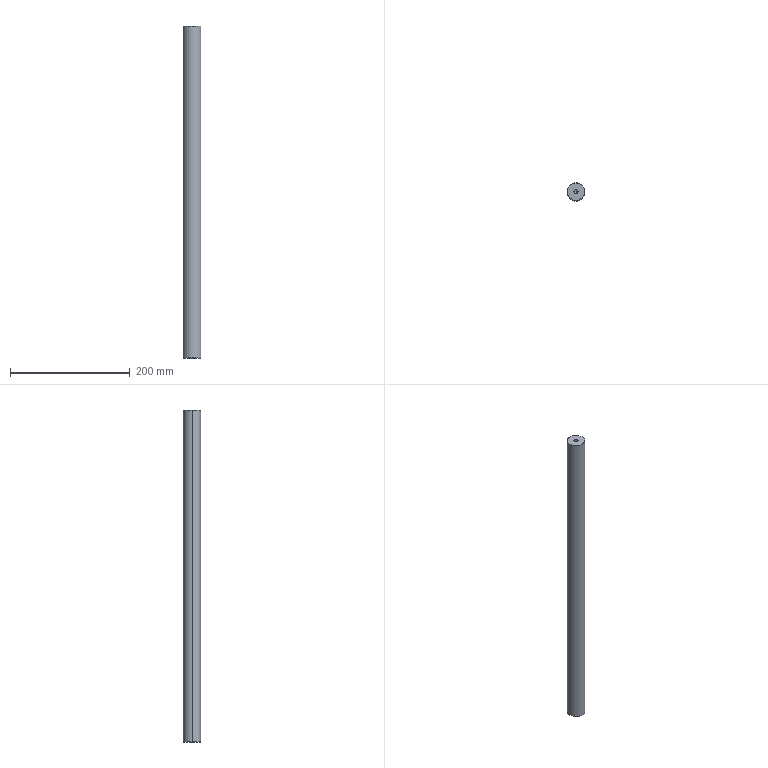Part | STEP file | 11-FG-SJ01511 | 1 solid | 16 faces | box 30 x 30 x 554 mm | volume 390089 mm3 | cone 8 | cylinder 6 | plane 2 | commonest cylinder face diameters 6.8 x4 30 x2
STEP:
#1=CARTESIAN_POINT('',(-14.5,0.,0.));
#2=VERTEX_POINT('',#1);
#3=CARTESIAN_POINT('',(14.5,0.,0.));
#4=VERTEX_POINT('',#3);
#5=CARTESIAN_POINT('',(0.,0.,0.));
#6=DIRECTION('',(0.,0.,-1.));
#7=DIRECTION('',(1.,0.,0.));
#8=AXIS2_PLACEMENT_3D('',#5,#6,#7);
#9=CIRCLE('',#8,14.5);
#10=EDGE_CURVE('',#2,#4,#9,.T.);
#11=ORIENTED_EDGE('',*,*,#10,.F.);
#12=CARTESIAN_POINT('',(-15.,0.,0.5));
#13=VERTEX_POINT('',#12);
#14=CARTESIAN_POINT('',(-15.,0.,0.5));
#15=DIRECTION('',(-0.7071,0.,0.7071));
#16=VECTOR('',#15,1000.);
#17=LINE('',#14,#16);
#18=EDGE_CURVE('',#2,#13,#17,.T.);
#19=ORIENTED_EDGE('',*,*,#18,.T.);
#20=CARTESIAN_POINT('',(15.,0.,0.5));
#21=VERTEX_POINT('',#20);
#22=CARTESIAN_POINT('',(0.,0.,0.5));
#23=DIRECTION('',(0.,0.,1.));
#24=DIRECTION('',(1.,0.,0.));
#25=AXIS2_PLACEMENT_3D('',#22,#23,#24);
#26=CIRCLE('',#25,15.);
#27=EDGE_CURVE('',#21,#13,#26,.T.);
#28=ORIENTED_EDGE('',*,*,#27,.F.);
#29=CARTESIAN_POINT('',(15.,0.,0.5));
#30=DIRECTION('',(0.7071,0.,0.7071));
#31=VECTOR('',#30,1000.);
#32=LINE('',#29,#31);
#33=EDGE_CURVE('',#4,#21,#32,.T.);
#34=ORIENTED_EDGE('',*,*,#33,.F.);
#35=EDGE_LOOP('',(#11,#19,#28,#34));
#36=FACE_OUTER_BOUND('',#35,.T.);
#37=CARTESIAN_POINT('',(0.,0.,0.5));
#38=DIRECTION('',(0.,0.,1.));
#39=DIRECTION('',(1.,0.,0.));
#40=AXIS2_PLACEMENT_3D('',#37,#38,#39);
#41=CONICAL_SURFACE('',#40,15.,0.7854);
#42=ADVANCED_FACE('',(#36),#41,.T.);
#43=CARTESIAN_POINT('',(14.5,0.,554.));
#44=VERTEX_POINT('',#43);
#45=CARTESIAN_POINT('',(-14.5,0.,554.));
#46=VERTEX_POINT('',#45);
#47=CARTESIAN_POINT('',(0.,0.,554.));
#48=DIRECTION('',(0.,0.,1.));
#49=DIRECTION('',(1.,0.,0.));
#50=AXIS2_PLACEMENT_3D('',#47,#48,#49);
#51=CIRCLE('',#50,14.5);
#52=EDGE_CURVE('',#44,#46,#51,.T.);
#53=ORIENTED_EDGE('',*,*,#52,.F.);
#54=CARTESIAN_POINT('',(15.,0.,553.5));
#55=VERTEX_POINT('',#54);
#56=CARTESIAN_POINT('',(14.5,0.,554.));
#57=DIRECTION('',(0.7071,0.,-0.7071));
#58=VECTOR('',#57,1000.);
#59=LINE('',#56,#58);
#60=EDGE_CURVE('',#44,#55,#59,.T.);
#61=ORIENTED_EDGE('',*,*,#60,.T.);
#62=CARTESIAN_POINT('',(-15.,0.,553.5));
#63=VERTEX_POINT('',#62);
#64=CARTESIAN_POINT('',(0.,0.,553.5));
#65=DIRECTION('',(0.,0.,-1.));
#66=DIRECTION('',(1.,0.,0.));
#67=AXIS2_PLACEMENT_3D('',#64,#65,#66);
#68=CIRCLE('',#67,15.);
#69=EDGE_CURVE('',#63,#55,#68,.T.);
#70=ORIENTED_EDGE('',*,*,#69,.F.);
#71=CARTESIAN_POINT('',(-14.5,0.,554.));
#72=DIRECTION('',(-0.7071,0.,-0.7071));
#73=VECTOR('',#72,1000.);
#74=LINE('',#71,#73);
#75=EDGE_CURVE('',#46,#63,#74,.T.);
#76=ORIENTED_EDGE('',*,*,#75,.F.);
#77=EDGE_LOOP('',(#53,#61,#70,#76));
#78=FACE_OUTER_BOUND('',#77,.T.);
#79=CARTESIAN_POINT('',(0.,0.,554.));
#80=DIRECTION('',(0.,0.,-1.));
#81=DIRECTION('',(-1.,0.,0.));
#82=AXIS2_PLACEMENT_3D('',#79,#80,#81);
#83=CONICAL_SURFACE('',#82,14.5,0.7854);
#84=ADVANCED_FACE('',(#78),#83,.T.);
#85=CARTESIAN_POINT('',(-3.4,0.,534.2));
#86=VERTEX_POINT('',#85);
#87=CARTESIAN_POINT('',(3.4,0.,534.2));
#88=VERTEX_POINT('',#87);
#89=CARTESIAN_POINT('',(0.,0.,534.2));
#90=DIRECTION('',(0.,0.,1.));
#91=DIRECTION('',(1.,0.,0.));
#92=AXIS2_PLACEMENT_3D('',#89,#90,#91);
#93=CIRCLE('',#92,3.4);
#94=EDGE_CURVE('',#86,#88,#93,.T.);
#95=ORIENTED_EDGE('',*,*,#94,.F.);
#96=CARTESIAN_POINT('',(-3.4,0.,554.));
#97=VERTEX_POINT('',#96);
#98=CARTESIAN_POINT('',(-3.4,0.,554.));
#99=DIRECTION('',(0.,0.,1.));
#100=VECTOR('',#99,1000.);
#101=LINE('',#98,#100);
#102=EDGE_CURVE('',#86,#97,#101,.T.);
#103=ORIENTED_EDGE('',*,*,#102,.T.);
#104=CARTESIAN_POINT('',(3.4,0.,554.));
#105=VERTEX_POINT('',#104);
#106=CARTESIAN_POINT('',(0.,0.,554.));
#107=DIRECTION('',(0.,0.,1.));
#108=DIRECTION('',(1.,0.,0.));
#109=AXIS2_PLACEMENT_3D('',#106,#107,#108);
#110=CIRCLE('',#109,3.4);
#111=EDGE_CURVE('',#97,#105,#110,.T.);
#112=ORIENTED_EDGE('',*,*,#111,.T.);
#113=CARTESIAN_POINT('',(3.4,0.,554.));
#114=DIRECTION('',(0.,0.,1.));
#115=VECTOR('',#114,1000.);
#116=LINE('',#113,#115);
#117=EDGE_CURVE('',#88,#105,#116,.T.);
#118=ORIENTED_EDGE('',*,*,#117,.F.);
#119=EDGE_LOOP('',(#95,#103,#112,#118));
#120=FACE_OUTER_BOUND('',#119,.T.);
#121=CARTESIAN_POINT('',(0.,0.,554.));
#122=DIRECTION('',(0.,0.,1.));
#123=DIRECTION('',(1.,0.,0.));
#124=AXIS2_PLACEMENT_3D('',#121,#122,#123);
#125=CYLINDRICAL_SURFACE('',#124,3.4);
#126=ADVANCED_FACE('',(#120),#125,.F.);
#127=CARTESIAN_POINT('',(0.,0.,532.157));
#128=VERTEX_POINT('',#127);
#129=CARTESIAN_POINT('',(3.4,0.,534.2));
#130=DIRECTION('',(0.8572,0.,0.515));
#131=VECTOR('',#130,1000.);
#132=LINE('',#129,#131);
#133=EDGE_CURVE('',#128,#88,#132,.T.);
#134=ORIENTED_EDGE('',*,*,#133,.F.);
#135=CARTESIAN_POINT('',(-3.4,0.,534.2));
#136=DIRECTION('',(-0.8572,0.,0.515));
#137=VECTOR('',#136,1000.);
#138=LINE('',#135,#137);
#139=EDGE_CURVE('',#128,#86,#138,.T.);
#140=ORIENTED_EDGE('',*,*,#139,.T.);
#141=ORIENTED_EDGE('',*,*,#94,.T.);
#142=EDGE_LOOP('',(#134,#140,#141));
#143=FACE_OUTER_BOUND('',#142,.T.);
#144=CARTESIAN_POINT('',(0.,0.,534.2));
#145=DIRECTION('',(0.,0.,1.));
#146=DIRECTION('',(1.,0.,0.));
#147=AXIS2_PLACEMENT_3D('',#144,#145,#146);
#148=CONICAL_SURFACE('',#147,3.4,1.03);
#149=ADVANCED_FACE('',(#143),#148,.F.);
#150=CARTESIAN_POINT('',(3.4,0.,19.8));
#151=VERTEX_POINT('',#150);
#152=CARTESIAN_POINT('',(-3.4,0.,19.8));
#153=VERTEX_POINT('',#152);
#154=CARTESIAN_POINT('',(0.,0.,19.8));
#155=DIRECTION('',(0.,0.,-1.));
#156=DIRECTION('',(-1.,0.,0.));
#157=AXIS2_PLACEMENT_3D('',#154,#155,#156);
#158=CIRCLE('',#157,3.4);
#159=EDGE_CURVE('',#151,#153,#158,.T.);
#160=ORIENTED_EDGE('',*,*,#159,.F.);
#161=CARTESIAN_POINT('',(3.4,0.,0.));
#162=VERTEX_POINT('',#161);
#163=CARTESIAN_POINT('',(3.4,0.,0.));
#164=DIRECTION('',(0.,0.,-1.));
#165=VECTOR('',#164,1000.);
#166=LINE('',#163,#165);
#167=EDGE_CURVE('',#151,#162,#166,.T.);
#168=ORIENTED_EDGE('',*,*,#167,.T.);
#169=CARTESIAN_POINT('',(-3.4,0.,0.));
#170=VERTEX_POINT('',#169);
#171=CARTESIAN_POINT('',(0.,0.,0.));
#172=DIRECTION('',(0.,0.,-1.));
#173=DIRECTION('',(-1.,0.,0.));
#174=AXIS2_PLACEMENT_3D('',#171,#172,#173);
#175=CIRCLE('',#174,3.4);
#176=EDGE_CURVE('',#162,#170,#175,.T.);
#177=ORIENTED_EDGE('',*,*,#176,.T.);
#178=CARTESIAN_POINT('',(-3.4,0.,0.));
#179=DIRECTION('',(0.,0.,-1.));
#180=VECTOR('',#179,1000.);
#181=LINE('',#178,#180);
#182=EDGE_CURVE('',#153,#170,#181,.T.);
#183=ORIENTED_EDGE('',*,*,#182,.F.);
#184=EDGE_LOOP('',(#160,#168,#177,#183));
#185=FACE_OUTER_BOUND('',#184,.T.);
#186=CARTESIAN_POINT('',(0.,0.,0.));
#187=DIRECTION('',(0.,0.,-1.));
#188=DIRECTION('',(-1.,0.,0.));
#189=AXIS2_PLACEMENT_3D('',#186,#187,#188);
#190=CYLINDRICAL_SURFACE('',#189,3.4);
#191=ADVANCED_FACE('',(#185),#190,.F.);
#192=CARTESIAN_POINT('',(0.,0.,21.843));
#193=VERTEX_POINT('',#192);
#194=CARTESIAN_POINT('',(-3.4,0.,19.8));
#195=DIRECTION('',(-0.8572,0.,-0.515));
#196=VECTOR('',#195,1000.);
#197=LINE('',#194,#196);
#198=EDGE_CURVE('',#193,#153,#197,.T.);
#199=ORIENTED_EDGE('',*,*,#198,.F.);
#200=CARTESIAN_POINT('',(3.4,0.,19.8));
#201=DIRECTION('',(0.8572,0.,-0.515));
#202=VECTOR('',#201,1000.);
#203=LINE('',#200,#202);
#204=EDGE_CURVE('',#193,#151,#203,.T.);
#205=ORIENTED_EDGE('',*,*,#204,.T.);
#206=ORIENTED_EDGE('',*,*,#159,.T.);
#207=EDGE_LOOP('',(#199,#205,#206));
#208=FACE_OUTER_BOUND('',#207,.T.);
#209=CARTESIAN_POINT('',(0.,0.,19.8));
#210=DIRECTION('',(0.,0.,-1.));
#211=DIRECTION('',(-1.,0.,0.));
#212=AXIS2_PLACEMENT_3D('',#209,#210,#211);
#213=CONICAL_SURFACE('',#212,3.4,1.03);
#214=ADVANCED_FACE('',(#208),#213,.F.);
#215=ORIENTED_EDGE('',*,*,#69,.T.);
#216=CARTESIAN_POINT('',(15.,0.,554.));
#217=DIRECTION('',(0.,0.,-1.));
#218=VECTOR('',#217,1000.);
#219=LINE('',#216,#218);
#220=EDGE_CURVE('',#55,#21,#219,.T.);
#221=ORIENTED_EDGE('',*,*,#220,.T.);
#222=ORIENTED_EDGE('',*,*,#27,.T.);
#223=CARTESIAN_POINT('',(-15.,0.,554.));
#224=DIRECTION('',(0.,0.,-1.));
#225=VECTOR('',#224,1000.);
#226=LINE('',#223,#225);
#227=EDGE_CURVE('',#63,#13,#226,.T.);
#228=ORIENTED_EDGE('',*,*,#227,.F.);
#229=EDGE_LOOP('',(#215,#221,#222,#228));
#230=FACE_OUTER_BOUND('',#229,.T.);
#231=CARTESIAN_POINT('',(0.,0.,554.));
#232=DIRECTION('',(0.,0.,-1.));
#233=DIRECTION('',(-1.,0.,0.));
#234=AXIS2_PLACEMENT_3D('',#231,#232,#233);
#235=CYLINDRICAL_SURFACE('',#234,15.);
#236=ADVANCED_FACE('',(#230),#235,.T.);
#237=ORIENTED_EDGE('',*,*,#220,.F.);
#238=CARTESIAN_POINT('',(0.,0.,553.5));
#239=DIRECTION('',(0.,0.,-1.));
#240=DIRECTION('',(1.,0.,0.));
#241=AXIS2_PLACEMENT_3D('',#238,#239,#240);
#242=CIRCLE('',#241,15.);
#243=EDGE_CURVE('',#55,#63,#242,.T.);
#244=ORIENTED_EDGE('',*,*,#243,.T.);
#245=ORIENTED_EDGE('',*,*,#227,.T.);
#246=CARTESIAN_POINT('',(0.,0.,0.5));
#247=DIRECTION('',(0.,0.,1.));
#248=DIRECTION('',(1.,0.,0.));
#249=AXIS2_PLACEMENT_3D('',#246,#247,#248);
#250=CIRCLE('',#249,15.);
#251=EDGE_CURVE('',#13,#21,#250,.T.);
#252=ORIENTED_EDGE('',*,*,#251,.T.);
#253=EDGE_LOOP('',(#237,#244,#245,#252));
#254=FACE_OUTER_BOUND('',#253,.T.);
#255=CARTESIAN_POINT('',(0.,0.,554.));
#256=DIRECTION('',(0.,0.,-1.));
#257=DIRECTION('',(-1.,0.,0.));
#258=AXIS2_PLACEMENT_3D('',#255,#256,#257);
#259=CYLINDRICAL_SURFACE('',#258,15.);
#260=ADVANCED_FACE('',(#254),#259,.T.);
#261=CARTESIAN_POINT('',(0.,0.,554.));
#262=DIRECTION('',(0.,0.,1.));
#263=DIRECTION('',(1.,0.,0.));
#264=AXIS2_PLACEMENT_3D('',#261,#262,#263);
#265=CIRCLE('',#264,14.5);
#266=EDGE_CURVE('',#46,#44,#265,.T.);
#267=ORIENTED_EDGE('',*,*,#266,.T.);
#268=ORIENTED_EDGE('',*,*,#52,.T.);
#269=EDGE_LOOP('',(#267,#268));
#270=FACE_OUTER_BOUND('',#269,.T.);
#271=CARTESIAN_POINT('',(0.,0.,554.));
#272=DIRECTION('',(0.,0.,1.));
#273=DIRECTION('',(1.,0.,0.));
#274=AXIS2_PLACEMENT_3D('',#271,#272,#273);
#275=CIRCLE('',#274,3.4);
#276=EDGE_CURVE('',#105,#97,#275,.T.);
#277=ORIENTED_EDGE('',*,*,#276,.F.);
#278=ORIENTED_EDGE('',*,*,#111,.F.);
#279=EDGE_LOOP('',(#277,#278));
#280=FACE_BOUND('',#279,.T.);
#281=CARTESIAN_POINT('',(0.,0.,554.));
#282=DIRECTION('',(0.,0.,1.));
#283=DIRECTION('',(1.,0.,0.));
#284=AXIS2_PLACEMENT_3D('',#281,#282,#283);
#285=PLANE('',#284);
#286=ADVANCED_FACE('',(#270,#280),#285,.T.);
#287=CARTESIAN_POINT('',(0.,0.,0.));
#288=DIRECTION('',(0.,0.,-1.));
#289=DIRECTION('',(1.,0.,0.));
#290=AXIS2_PLACEMENT_3D('',#287,#288,#289);
#291=CIRCLE('',#290,14.5);
#292=EDGE_CURVE('',#4,#2,#291,.T.);
#293=ORIENTED_EDGE('',*,*,#292,.T.);
#294=ORIENTED_EDGE('',*,*,#10,.T.);
#295=EDGE_LOOP('',(#293,#294));
#296=FACE_OUTER_BOUND('',#295,.T.);
#297=CARTESIAN_POINT('',(0.,0.,0.));
#298=DIRECTION('',(0.,0.,-1.));
#299=DIRECTION('',(-1.,0.,0.));
#300=AXIS2_PLACEMENT_3D('',#297,#298,#299);
#301=CIRCLE('',#300,3.4);
#302=EDGE_CURVE('',#170,#162,#301,.T.);
#303=ORIENTED_EDGE('',*,*,#302,.F.);
#304=ORIENTED_EDGE('',*,*,#176,.F.);
#305=EDGE_LOOP('',(#303,#304));
#306=FACE_BOUND('',#305,.T.);
#307=CARTESIAN_POINT('',(0.,0.,0.));
#308=DIRECTION('',(0.,0.,1.));
#309=DIRECTION('',(1.,0.,0.));
#310=AXIS2_PLACEMENT_3D('',#307,#308,#309);
#311=PLANE('',#310);
#312=ADVANCED_FACE('',(#296,#306),#311,.F.);
#313=ORIENTED_EDGE('',*,*,#204,.F.);
#314=ORIENTED_EDGE('',*,*,#198,.T.);
#315=CARTESIAN_POINT('',(0.,0.,19.8));
#316=DIRECTION('',(0.,0.,-1.));
#317=DIRECTION('',(-1.,0.,0.));
#318=AXIS2_PLACEMENT_3D('',#315,#316,#317);
#319=CIRCLE('',#318,3.4);
#320=EDGE_CURVE('',#153,#151,#319,.T.);
#321=ORIENTED_EDGE('',*,*,#320,.T.);
#322=EDGE_LOOP('',(#313,#314,#321));
#323=FACE_OUTER_BOUND('',#322,.T.);
#324=CARTESIAN_POINT('',(0.,0.,19.8));
#325=DIRECTION('',(0.,0.,-1.));
#326=DIRECTION('',(-1.,0.,0.));
#327=AXIS2_PLACEMENT_3D('',#324,#325,#326);
#328=CONICAL_SURFACE('',#327,3.4,1.03);
#329=ADVANCED_FACE('',(#323),#328,.F.);
#330=ORIENTED_EDGE('',*,*,#167,.F.);
#331=ORIENTED_EDGE('',*,*,#320,.F.);
#332=ORIENTED_EDGE('',*,*,#182,.T.);
#333=ORIENTED_EDGE('',*,*,#302,.T.);
#334=EDGE_LOOP('',(#330,#331,#332,#333));
#335=FACE_OUTER_BOUND('',#334,.T.);
#336=CARTESIAN_POINT('',(0.,0.,0.));
#337=DIRECTION('',(0.,0.,-1.));
#338=DIRECTION('',(-1.,0.,0.));
#339=AXIS2_PLACEMENT_3D('',#336,#337,#338);
#340=CYLINDRICAL_SURFACE('',#339,3.4);
#341=ADVANCED_FACE('',(#335),#340,.F.);
#342=ORIENTED_EDGE('',*,*,#139,.F.);
#343=ORIENTED_EDGE('',*,*,#133,.T.);
#344=CARTESIAN_POINT('',(0.,0.,534.2));
#345=DIRECTION('',(0.,0.,1.));
#346=DIRECTION('',(1.,0.,0.));
#347=AXIS2_PLACEMENT_3D('',#344,#345,#346);
#348=CIRCLE('',#347,3.4);
#349=EDGE_CURVE('',#88,#86,#348,.T.);
#350=ORIENTED_EDGE('',*,*,#349,.T.);
#351=EDGE_LOOP('',(#342,#343,#350));
#352=FACE_OUTER_BOUND('',#351,.T.);
#353=CARTESIAN_POINT('',(0.,0.,534.2));
#354=DIRECTION('',(0.,0.,1.));
#355=DIRECTION('',(1.,0.,0.));
#356=AXIS2_PLACEMENT_3D('',#353,#354,#355);
#357=CONICAL_SURFACE('',#356,3.4,1.03);
#358=ADVANCED_FACE('',(#352),#357,.F.);
#359=ORIENTED_EDGE('',*,*,#102,.F.);
#360=ORIENTED_EDGE('',*,*,#349,.F.);
#361=ORIENTED_EDGE('',*,*,#117,.T.);
#362=ORIENTED_EDGE('',*,*,#276,.T.);
#363=EDGE_LOOP('',(#359,#360,#361,#362));
#364=FACE_OUTER_BOUND('',#363,.T.);
#365=CARTESIAN_POINT('',(0.,0.,554.));
#366=DIRECTION('',(0.,0.,1.));
#367=DIRECTION('',(1.,0.,0.));
#368=AXIS2_PLACEMENT_3D('',#365,#366,#367);
#369=CYLINDRICAL_SURFACE('',#368,3.4);
#370=ADVANCED_FACE('',(#364),#369,.F.);
#371=ORIENTED_EDGE('',*,*,#60,.F.);
#372=ORIENTED_EDGE('',*,*,#266,.F.);
#373=ORIENTED_EDGE('',*,*,#75,.T.);
#374=ORIENTED_EDGE('',*,*,#243,.F.);
#375=EDGE_LOOP('',(#371,#372,#373,#374));
#376=FACE_OUTER_BOUND('',#375,.T.);
#377=CARTESIAN_POINT('',(0.,0.,554.));
#378=DIRECTION('',(0.,0.,-1.));
#379=DIRECTION('',(-1.,0.,0.));
#380=AXIS2_PLACEMENT_3D('',#377,#378,#379);
#381=CONICAL_SURFACE('',#380,14.5,0.7854);
#382=ADVANCED_FACE('',(#376),#381,.T.);
#383=ORIENTED_EDGE('',*,*,#18,.F.);
#384=ORIENTED_EDGE('',*,*,#292,.F.);
#385=ORIENTED_EDGE('',*,*,#33,.T.);
#386=ORIENTED_EDGE('',*,*,#251,.F.);
#387=EDGE_LOOP('',(#383,#384,#385,#386));
#388=FACE_OUTER_BOUND('',#387,.T.);
#389=CARTESIAN_POINT('',(0.,0.,0.5));
#390=DIRECTION('',(0.,0.,1.));
#391=DIRECTION('',(1.,0.,0.));
#392=AXIS2_PLACEMENT_3D('',#389,#390,#391);
#393=CONICAL_SURFACE('',#392,15.,0.7854);
#394=ADVANCED_FACE('',(#388),#393,.T.);
#395=CLOSED_SHELL('',(#42,#84,#126,#149,#191,#214,#236,#260,#286,#312,#329,#341,#358,#370,#382,#394));
#396=MANIFOLD_SOLID_BREP('',#395);
#397=CARTESIAN_POINT('',(0.,0.,0.));
#398=DIRECTION('',(0.,0.,1.));
#399=DIRECTION('',(1.,0.,0.));
#400=AXIS2_PLACEMENT_3D('',#397,#398,#399);
#401=(LENGTH_UNIT()NAMED_UNIT(*)SI_UNIT(.MILLI.,.METRE.));
#402=UNCERTAINTY_MEASURE_WITH_UNIT(LENGTH_MEASURE(0.00001),#401,'','');
#403=(NAMED_UNIT(*)PLANE_ANGLE_UNIT()SI_UNIT($,.RADIAN.));
#404=(NAMED_UNIT(*)SI_UNIT($,.STERADIAN.)SOLID_ANGLE_UNIT());
#405=(GEOMETRIC_REPRESENTATION_CONTEXT(3)GLOBAL_UNCERTAINTY_ASSIGNED_CONTEXT((#402))GLOBAL_UNIT_ASSIGNED_CONTEXT((#401,#403,#404))REPRESENTATION_CONTEXT('',''));
#406=ADVANCED_BREP_SHAPE_REPRESENTATION('',(#396,#400),#405);